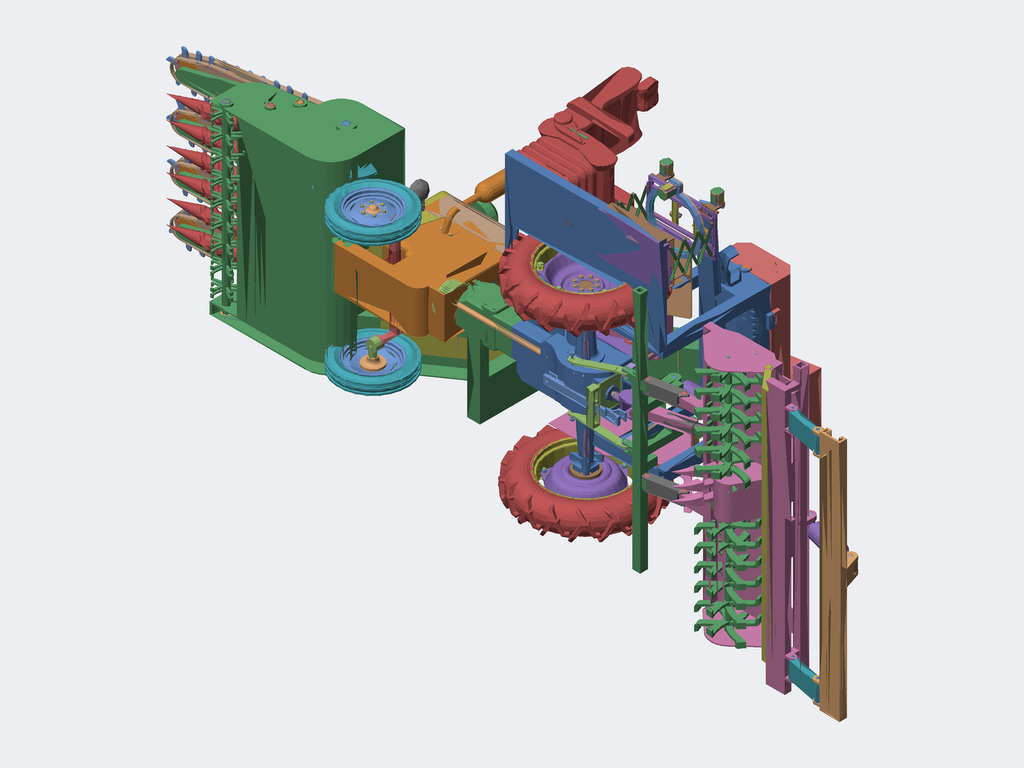Assembly | SolidWorks | 153 different items | 1051 placed
Parts list (item | name | quantity | parent item | size | volume):
1 | (subassembly) | x1 | - | - | 16381446 mm3
2 | (subassembly) | x89 | - | 79.994 x 100.305 x 21.303 mm | 62086 mm3
3 | (subassembly) | x89 | - | 59.12 x 16 x 20 mm | 6391 mm3
4 | - | x1 | - | 480 x 80 x 140 mm | 1729991 mm3
5 | - | x2 | - | 65 x 16 x 16 mm | 12827 mm3
6 | - | x2 | - | 70 x 20 x 20 mm | 21455 mm3
7 | - | x1 | - | 10 x 70 x 330 mm | 231000 mm3
8 | - | x10 | - | 25.3 x 15.011 x 13 mm | 1760 mm3
9 | - | x1 | - | 40 x 40 x 80 mm | 43982 mm3
10 | - | x2 | - | 435 x 150 x 150 mm | 3088587 mm3
11 | - | x2 | - | 380 x 110 x 110 mm | 1045872 mm3
12 | - | x1 | - | 1433 x 943.59 x 2500 mm | 127808893 mm3
13 | - | x1 | - | 50 x 305 x 2270 mm | 21360963 mm3
14 | - | x2 | - | 36 x 40 x 318 mm | 121648 mm3
15 | - | x89 | in 2 | 36.56 x 20 x 100 mm | 55695 mm3
16 | - | x1 | - | 44.721 x 70 x 40 mm | 80979 mm3
17 | - | x1 | - | 30 x 30 x 120 mm | 84731 mm3
18 | - | x1 | - | 40 x 120 x 40 mm | 150673 mm3
19 | - | x4 | - | 40 x 110 x 40 mm | 138107 mm3
20 | - | x1 | - | 50 x 150 x 50 mm | 293913 mm3
21 | - | x1 | - | 40 x 150 x 40 mm | 187421 mm3
22 | - | x4 | - | 30 x 30 x 200 mm | 141280 mm3
23 | - | x2 | - | 372 x 72 x 110 mm | 2095609 mm3
24 | - | x2 | - | 360 x 60 x 160 mm | 3106195 mm3
25 | - | x1 | - | 275 x 250 x 2300 mm | 16623350 mm3
26 | - | x2 | - | 39.6 x 34.295 x 22.3 mm | 15063 mm3
27 | - | x1 | in 1 | 25 x 25 x 230 mm | 40077 mm3
28 | - | x4 | in 1 | - | -
29 | - | x2 | in 1 | 150 x 115 x 15 mm | 137970 mm3
30 | - | x4 | in 1 | 60 x 60 x 8 mm | 18784 mm3
31 | - | x4 | in 1 | 15 x 15 x 35.5 mm | 2158 mm3
32 | - | x4 | in 1 | 60 x 10 x 10 mm | 2893 mm3
33 | - | x1 | in 1 | 605.5 x 531 x 90 mm | 1417338 mm3
34 | - | x1 | in 1 | 507.991 x 507.957 x 60 mm | 736026 mm3
35 | - | x2 | in 1 | 15 x 10 x 574 mm | 77716 mm3
36 | - | x1 | in 1 | 87.341 x 87.341 x 20 mm | 92376 mm3
37 | - | x2 | - | 130 x 50 x 50 mm | 156637 mm3
38 | - | x1 | in 1 | 634 x 120 x 390 mm | 7186342 mm3
39 | - | x1 | in 1 | 120 x 95 x 15 mm | 107220 mm3
40 | - | x1 | - | 766.626 x 1417 x 630 mm | 182133754 mm3
41 | - | x2 | in 1 | 43 x 45 x 33 mm | 8145 mm3
42 | - | x2 | in 1 | 43 x 45 x 33 mm | 8145 mm3
43 | - | x2 | in 1 | 54 x 50 x 30 mm | 26614 mm3
44 | - | x2 | in 1 | 54 x 10 x 290 mm | 145188 mm3
45 | - | x4 | in 1 | - | -
46 | - | x8 | in 1 | 32 x 12 x 33.1 mm | 9311 mm3
47 | - | x1 | - | - | -
48 | - | x2 | - | 47 x 47 x 5 mm | 6107 mm3
49 | - | x2 | in 1 | 15 x 10 x 240 mm | 32544 mm3
50 | - | x2 | in 1 | 25 x 70 x 35 mm | 25493 mm3
51 | - | x1 | in 1 | 634 x 60 x 390 mm | 1783210 mm3
52 | - | x10 | - | 82 x 50 x 50 mm | 78196 mm3
53 | - | x10 | - | 112.877 x 112.877 x 35 mm | 271354 mm3
54 | - | x20 | in 1 | 24 x 14 x 14 mm | 2187 mm3
55 | - | x2 | in 1 | 25 x 180 x 20 mm | 48842 mm3
56 | - | x1 | in 1 | 20 x 20 x 638 mm | 238279 mm3
57 | - | x12 | in 1 | 20 x 321 x 10 mm | 60985 mm3
58 | - | x12 | - | 179.981 x 179.731 x 50 mm | 415384 mm3
59 | - | x178 | in 2, 3 | 37.56 x 16 x 15 mm | 3392 mm3
60 | - | x178 | in 2, 3 | 37.56 x 16 x 20 mm | 2999 mm3
61 | - | x1 | - | 232.128 x 238.99 x 1760 mm | 6921520 mm3
62 | - | x6 | - | - | 6506170 mm3
63 | - | x1 | - | 547.5 x 225 x 360 mm | 8692071 mm3
64 | - | x1 | - | 40 x 40 x 1760 mm | 1700428 mm3
65 | - | x4 | - | 105 x 40 x 40 mm | 98226 mm3
66 | - | x1 | - | 40 x 40 x 1760 mm | 1776548 mm3
67 | - | x3 | - | 80 x 80 x 20 mm | 63234 mm3
68 | - | x1 | - | 70 x 95.558 x 40 mm | 119109 mm3
69 | - | x1 | - | 90 x 20 x 90 mm | 78186 mm3
70 | - | x4 | - | 280 x 100 x 1224 mm | 5139884 mm3
71 | - | x1 | - | 315 x 60 x 325 mm | 1362122 mm3
72 | - | x1 | - | 1005 x 380.05 x 470 mm | 23114578 mm3
73 | - | x1 | - | 1490 x 380.05 x 2280 mm | 110050960 mm3
74 | - | x1 | - | 387.638 x 226.527 x 70 mm | 165213 mm3
75 | - | x1 | - | 381.145 x 360 x 307.969 mm | 3545128 mm3
76 | - | x1 | - | 374.894 x 400 x 497.382 mm | 13317913 mm3
77 | - | x1 | - | 1005 x 791.422 x 614.545 mm | 64772988 mm3
78 | - | x2 | - | 94 x 45 x 55 mm | 48372 mm3
79 | - | x2 | - | 652 x 122 x 652 mm | 6413789 mm3
80 | - | x2 | - | 100 x 170 x 370 mm | 1067997 mm3
81 | - | x2 | - | 100 x 270 x 310 mm | 1436503 mm3
82 | - | x1 | - | 248.057 x 1018 x 150 mm | 2628075 mm3
83 | - | x1 | - | 420 x 110 x 420 mm | 545281 mm3
84 | - | x2 | - | 161 x 220.5 x 101.1 mm | 223051 mm3
85 | - | x1 | - | 153.486 x 153.486 x 325.608 mm | 831676 mm3
86 | - | x2 | - | 32.5 x 20.785 x 18 mm | 4879 mm3
87 | - | x1 | - | 510 x 325.072 x 1140 mm | 2882610 mm3
88 | - | x1 | - | 500 x 154.34 x 530 mm | 1123560 mm3
89 | - | x1 | - | 1070 x 600 x 360 mm | 4618746 mm3
90 | - | x2 | - | 244.595 x 1180 x 1180 mm | 23262229 mm3
91 | - | x2 | - | 180 x 105 x 180 mm | 867546 mm3
92 | - | x2 | - | 748.86 x 226.672 x 748.86 mm | 3116761 mm3
93 | - | x2 | - | 593.907 x 665 x 128.5 mm | 2994623 mm3
94 | - | x2 | - | 218 x 130 x 218 mm | 1192193 mm3
95 | - | x1 | - | 1070 x 600 x 360 mm | 3106000 mm3
96 | - | x2 | - | 458.731 x 420 x 1075 mm | 11323145 mm3
97 | - | x4 | - | 15 x 68 x 68 mm | 23045 mm3
98 | - | x6 | - | 12 x 60 x 60 mm | 12840 mm3
99 | - | x1 | - | 211.926 x 211.926 x 276.87 mm | 1401987 mm3
100 | - | x2 | - | 252.245 x 252.245 x 629.793 mm | 2125669 mm3
101 | - | x1 | - | 40 x 40 x 1385 mm | 1706048 mm3
102 | - | x1 | - | 209.617 x 209.617 x 100 mm | 2166914 mm3
103 | - | x2 | - | 96.667 x 455.608 x 455.608 mm | 1172743 mm3
104 | - | x1 | - | 309.756 x 309.756 x 100 mm | 4555207 mm3
105 | - | x1 | - | 435.01 x 940 x 945 mm | 125087598 mm3
106 | - | x1 | - | 530 x 40 x 400 mm | 7871394 mm3
107 | - | x1 | - | 153.486 x 153.486 x 294.64 mm | 719014 mm3
108 | - | x6 | - | 12 x 62 x 62 mm | 13593 mm3
109 | - | x1 | - | 290 x 322.5 x 290 mm | 420186 mm3
110 | - | x1 | - | 40 x 40 x 170 mm | 184147 mm3
111 | - | x1 | - | 250 x 228 x 335 mm | 4838196 mm3
112 | - | x1 | - | 490 x 137.955 x 138 mm | 3818604 mm3
113 | - | x1 | - | 12 x 42 x 42 mm | 7887 mm3
114 | - | x1 | - | 167.128 x 160.8 x 40 mm | 32904 mm3
115 | - | x1 | - | 80 x 330 x 830 mm | 1520421 mm3
116 | - | x1 | - | 70 x 218 x 225.232 mm | 296939 mm3
117 | - | x1 | - | 60 x 218 x 225.232 mm | 538282 mm3
118 | - | x2 | - | 140 x 120 x 290 mm | 1506174 mm3
119 | - | x1 | - | 1500 x 530.531 x 580 mm | 26783314 mm3
120 | - | x1 | - | 540 x 1030 x 1860 mm | 48317416 mm3
121 | - | x1 | - | 385.062 x 400 x 1200 mm | 5164108 mm3
122 | - | x1 | - | 4060 x 1991 x 1785 mm | 166702923 mm3
123 | - | x1 | - | 480.011 x 480.011 x 1760 mm | 34687851 mm3
124 | - | x6 | - | 7 x 65 x 65 mm | 6140 mm3
125 | - | x4 | - | 7 x 32 x 32 mm | 2319 mm3
126 | - | x2 | - | 40 x 40 x 415 mm | 466608 mm3
127 | - | x1 | - | 710 x 70 x 85 mm | 1467586 mm3
128 | - | x2 | - | 255 x 41.569 x 36 mm | 118287 mm3
129 | - | x2 | - | 55 x 140 x 140 mm | 524256 mm3
130 | - | x2 | - | 24 x 2.5 x 24 mm | 784.672 mm3
131 | - | x2 | - | 37 x 3 x 37 mm | 2154 mm3
132 | - | x10 | - | 20 x 2 x 20 mm | 427.568 mm3
133 | - | x4 | - | 77.7 x 43 x 43 mm | 30766 mm3
134 | - | x4 | - | 25.5 x 17.5 x 17.5 mm | 2396 mm3
135 | - | x12 | - | 23.7 x 23.7 x 3 mm | 898.415 mm3
136 | - | x12 | - | 18 x 20.785 x 12 mm | 2348 mm3
137 | - | x28 | - | 38.4 x 38.4 x 4 mm | 3151 mm3
138 | - | x16 | - | 24 x 27.713 x 16.4 mm | 5589 mm3
139 | - | x2 | - | 510.518 x 105 x 65 mm | 489274 mm3
140 | - | x1 | - | 480 x 80 x 140 mm | 1449991 mm3
141 | - | x14 | - | 33 x 28.579 x 19 mm | 8913 mm3
142 | - | x12 | - | 92.5 x 34.641 x 30 mm | 34747 mm3
143 | - | x4 | - | 70 x 70 x 30 mm | 65058 mm3
144 | - | x1 | - | 510 x 622 x 2300 mm | 17041991 mm3
145 | - | x1 | - | 100 x 99.955 x 305 mm | 1401130 mm3
146 | - | x1 | - | 180 x 165 x 210 mm | 1913564 mm3
147 | - | x2 | - | 150 x 20 x 150 mm | 232085 mm3
148 | - | x2 | - | 70 x 70 x 20 mm | 49524 mm3
149 | - | x2 | - | 52.5 x 34.641 x 30 mm | 22112 mm3
150 | - | x2 | - | 387.698 x 79.396 x 190 mm | 762316 mm3
151 | - | x1 | - | 593 x 758 x 290 mm | 1986947 mm3
152 | plain washers--product grade c gb | x1 | - | - | -
153 | prevailing torque all-metal 1 gb | x1 | - | - | -
Mates (type | each side: item.copy, entity, surface, feature), first 556 of 812 lines:
In the top assembly
Coincident | 73.1 face plane Boss-Extrude 1 | 77.1 face plane Boss-Extrude 1 | 2 times
Coincident | 73.1 face plane Cut-Extrude 1 | 77.1 face plane Boss-Extrude 1
Coincident | 105.1 face plane Cut-Extrude 1 | 77.1 face plane Boss-Extrude 7 | 2 times
Coincident | 105.1 edge | 77.1 face plane Boss-Extrude 7
Concentric | 105.1 face cylinder Boss-Extrude 11 | 115.1 face cylinder Boss-Extrude 2
Coincident | 105.1 face plane Boss-Extrude 1 | 115.1 face plane Boss-Extrude 2
Parallel | 105.1 face plane Boss-Extrude 13 | 115.1 face plane Extrude-Thin 3
Coincident | 73.1 face plane Boss-Extrude 1 | 63.1 face plane Boss-Extrude 1
Coincident | 73.1 face plane Boss-Extrude 1 | 63.1 face plane Boss-Extrude 3 | 2 times
Coincident | 73.1 face plane Boss-Extrude 1 | 75.1 face plane Boss-Extrude 2
Coincident | 73.1 face plane Cut-Extrude 1 | 75.1 face plane Boss-Extrude 2
Coincident | 63.1 face plane Boss-Extrude 1 | 75.1 face plane Boss-Extrude 2
Width | 76.1 face plane Boss-Extrude 4 | 76.1 face plane Boss-Extrude 4 | 63.1 face plane Mirror 2 | 63.1 face plane Boss-Extrude 2
Coincident | 63.1 face plane Boss-Extrude 1 | 76.1 face plane Boss-Extrude 4 | 2 times
Concentric | 105.1 face cylinder Boss-Extrude 4 | 106.1 face cylinder Cut-Extrude 3
Coincident | 105.1 face plane Boss-Extrude 3 | 106.1 face plane Cut-Extrude 4
LimitPlanarAngleDim | 105.1 face plane Boss-Extrude 1 | 106.1 face plane Boss-Extrude 1
Concentric | 91.1 face cylinder Revolve 1 | 103.1 face cylinder Thicken 2
Concentric | 91.1 face cylinder Boss-Extrude 1 | 103.1 face cylinder Cut-Extrude 1
Coincident | 91.1 face plane Revolve 1 | 103.1 face plane Thicken 2
Concentric | 79.1 face cylinder Thicken 1 | 103.1 face cylinder Thicken 1
Width | 103.1 face plane Thicken 1 | 103.1 face plane Thicken 1 | 79.1 face plane Thicken 1 | 79.1 face plane Thicken 1
Concentric | 80.1 face cylinder Boss-Extrude 3 | 81.1 face cylinder Cut-Extrude 1
Coincident | 80.1 edge | 81.1 face plane Revolve 1
Coincident | 91.1 face plane Revolve 1 | 80.1 face plane Boss-Extrude 1
Concentric | 91.1 face cylinder Revolve 1 | 80.1 face cylinder Boss-Extrude 1
Concentric | 115.1 face cylinder Extrude-Thin 1 | 81.1 face cylinder Boss-Extrude 1
LimitDistanceDim | 81.1 face plane Boss-Extrude 1 | 115.1 face plane Extrude-Thin 1
Parallel | 105.1 face plane Boss-Extrude 13 | 80.1 face plane Boss-Extrude 3
Coincident | 77.1 edge | 83.1 face plane CirPattern 1
Concentric | 77.1 face cylinder Boss-Extrude 6 | 83.1 face cylinder CirPattern 1
Coincident | 151.1 face plane Boss-Extrude 1 | 87.1 face plane Boss-Extrude 1
Concentric | 151.1 face cylinder Fillet 2 | 87.1 face cylinder Boss-Extrude 1
Coincident | 151.1 face plane Cut-Extrude 1 | 87.1 face plane Boss-Extrude 1
Concentric | 87.1 face cylinder Boss-Extrude 1 | 88.1 face cylinder Fillet 1 | 2 times
Coincident | 87.1 face plane Boss-Extrude 1 | 88.1 face plane Boss-Extrude 1
Width | 88.1 face plane Boss-Extrude 1 | 88.1 face plane Boss-Extrude 1 | 73.1 face plane Cut-Extrude 1 | 73.1 face plane Mirror 1
Coincident | 88.1 face plane Cut-Extrude 4 | 73.1 face plane Boss-Extrude 1
Coincident | 75.1 face plane Boss-Extrude 2 | 88.1 edge
Parallel | 105.1 face plane Boss-Extrude 1 | 91.1 face plane Revolve 1
Concentric | 81.2 face cylinder Revolve 1 | 80.2 face cylinder Boss-Extrude 3
Coincident | 81.2 face plane Revolve 1 | 80.2 face plane Boss-Extrude 2
Concentric | 115.1 face cylinder Extrude-Thin 1 | 81.2 face cylinder Boss-Extrude 1
LimitDistanceDim | 115.1 face plane Extrude-Thin 1 | 81.2 face plane Boss-Extrude 1
Parallel | 105.1 face plane Boss-Extrude 13 | 80.2 face plane Boss-Extrude 3
Concentric | 80.2 face cylinder Boss-Extrude 1 | 91.2 face cylinder Revolve 1
Coincident | 80.2 face plane Boss-Extrude 1 | 91.2 face plane Revolve 1
Parallel | 105.1 face plane Boss-Extrude 1 | 91.2 face plane Revolve 1
Concentric | 103.2 edge | 91.2 face cylinder Revolve 1
Concentric | 103.2 face cylinder CirPattern 1 | 91.2 face cylinder CirPattern 1
Coincident | 103.2 face plane Thicken 2 | 91.2 face plane Revolve 1
Width | 103.2 face plane Thicken 1 | 103.2 face plane Thicken 1 | 79.2 face plane Thicken 1 | 79.2 face plane Thicken 1
Concentric | 79.2 face cylinder Thicken 1 | 103.2 face cylinder Thicken 1
Concentric | 105.1 edge | 82.1 face cylinder Boss-Extrude 2
Coincident | 105.1 edge | 82.1 face cylinder Boss-Extrude 2
Coincident | 105.1 face plane Boss-Extrude 1 | 82.1 face plane Boss-Extrude 2
Concentric | 105.1 face cylinder Cut-Extrude 14 | 109.1 face cylinder Boss-Extrude 1 | 2 times
Coincident | 105.1 face plane Boss-Extrude 7 | 109.1 face plane Boss-Extrude 1
Concentric | 93.1 face cylinder Thicken 1 | 94.1 edge
Coincident | 93.1 face plane Thicken 1 | 94.1 face plane Revolve 1
Concentric | 93.1 face cylinder CirPattern 2 | 94.1 face cylinder CirPattern 1
Concentric | 94.2 face cylinder Revolve 1 | 93.2 face cylinder Thicken 1
Coincident | 94.2 face plane Revolve 1 | 93.2 face plane Thicken 1
Concentric | 94.2 face cylinder CirPattern 1 | 93.2 face cylinder CirPattern 2
Coincident | 94.1 face plane Boss-Extrude 2 | 100.1 face plane Cut-Extrude 1
Concentric | 94.1 face cylinder Revolve 1 | 100.1 face cylinder Boss-Extrude 1
Coincident | 94.1 face plane Revolve 1 | 100.1 face plane Boss-Extrude 1
Concentric | 94.2 face cylinder Revolve 1 | 100.2 face cylinder Boss-Extrude 1
Coincident | 94.2 face plane Boss-Extrude 2 | 100.2 face plane Cut-Extrude 1
Coincident | 94.2 face plane Revolve 1 | 100.2 edge
Concentric | 73.1 face cylinder Cut-Extrude 2 | 100.2 face cylinder Boss-Extrude 1
Concentric | 73.1 face cylinder Cut-Extrude 2 | 100.1 face cylinder Boss-Extrude 1
Concentric | 98.1 face cylinder Boss-Revolve 4 | 98.2 face cylinder Boss-Revolve 4
Concentric | 100.1 face cylinder Boss-Extrude 1 | 98.2 face cylinder Boss-Revolve 4
Coincident | 100.1 face plane Boss-Extrude 3 | 98.1 face plane Mirror All 1
Coincident | 100.1 face plane Boss-Extrude 2 | 98.2 face plane Boss-Revolve 4
Concentric | 98.3 face cylinder Boss-Revolve 4 | 98.4 face cylinder Boss-Revolve 4
Concentric | 100.2 face cylinder Boss-Extrude 1 | 98.4 face cylinder Boss-Revolve 3
Coincident | 100.2 edge | 98.3 face plane Boss-Revolve 4
Coincident | 100.2 face plane Boss-Extrude 2 | 98.4 edge
Coincident | 73.1 face plane Mirror 1 | 94.2 face plane Revolve 1
Coincident | 73.1 face plane Boss-Extrude 10 | 94.1 face plane Revolve 1
Concentric | 73.1 face cylinder Cut-Extrude 6 | 99.1 face cylinder Boss-Extrude 1
Concentric | 73.1 face cylinder Boss-Extrude 15 | 97.1 face cylinder Boss-Revolve 4
Coincident | 73.1 face plane Shell 1 | 97.1 face plane Mirror All 1
Coincident | 99.1 face plane Cut-Extrude 1 | 101.1 face plane Boss-Extrude 5 | 2 times
Concentric | 99.1 face cylinder Cut-Extrude 1 | 101.1 face cylinder Boss-Extrude 2
Concentric | 101.1 face cylinder Boss-Extrude 2 | 97.2 face cylinder Boss-Revolve 3
Coincident | 77.1 face plane Cut-Extrude 3 | 97.2 face plane Mirror All 1
Concentric | 101.1 face cylinder Boss-Extrude 2 | 98.5 face cylinder Boss-Revolve 3
Coincident | 105.1 edge | 98.5 face plane Mirror All 1
Concentric | 105.1 face cylinder Cut-Extrude 16 | 98.6 face cylinder Mirror All 1
Coincident | 105.1 face plane Extrude-Thin 3 | 98.6 face plane Mirror All 1
Concentric | 105.1 face cylinder Cut-Extrude 16 | 98.6 face cylinder Boss-Revolve 4
Coincident | 101.1 face plane Boss-Extrude 3 | 104.1 face plane Cut-Extrude 2
Concentric | 101.1 face cylinder Boss-Extrude 2 | 104.1 face cylinder Cut-Extrude 2
Coincident | 101.1 edge | 104.1 face plane SpurGear2
Concentric | 105.1 face cylinder Boss-Extrude 6 | 102.1 face cylinder Cut-Extrude 1
Coincident | 102.1 face plane SpurGear1 | 104.1 face plane SpurGear2
GearDim | 104.1 edge | 102.1 edge
Concentric | 108.1 face cylinder Boss-Revolve 4 | 108.2 face cylinder Boss-Revolve 4
Coincident | 102.1 face plane Cut-Extrude 1 | 108.2 face plane Boss-Revolve 4
Concentric | 102.1 face cylinder Cut-Extrude 1 | 108.2 face cylinder Boss-Revolve 3
Coincident | 102.1 face plane SpurGear1 | 108.1 face plane Boss-Revolve 3
Coincident | 105.1 face plane Boss-Extrude 6 | 102.1 face plane Cut-Extrude 1
Concentric | 111.1 face cylinder Cut-Extrude 5 | 112.1 face cylinder Revolve 1
Coincident | 111.1 face plane Boss-Extrude 3 | 112.1 face plane Revolve 1
Concentric | 112.1 face cylinder Revolve 1 | 113.1 face cylinder Boss-Revolve 4
Coincident | 111.1 face plane Boss-Extrude 1 | 113.1 face plane Boss-Revolve 4
Concentric | 112.1 face cylinder Revolve 1 | 114.1 face cylinder Boss-Extrude 1
Coincident | 112.1 face plane Cut-Extrude 3 | 114.1 face plane Boss-Extrude 3
Coincident | 112.1 face plane Revolve 1 | 114.1 face plane Boss-Extrude 2
Concentric | 111.1 face cylinder Boss-Extrude 1 | 116.1 face cylinder Thicken 1
Concentric | 111.1 face cylinder CirPattern 2 | 116.1 face cylinder CirPattern 1
Coincident | 111.1 face plane Boss-Extrude 1 | 116.1 face plane Thicken 1
Concentric | 111.1 face cylinder Boss-Extrude 1 | 117.1 face cylinder Thicken 1
Concentric | 111.1 face cylinder CirPattern 3 | 117.1 face cylinder CirPattern 4
Coincident | 111.1 face plane Boss-Extrude 1 | 117.1 face plane Thicken 1
Concentric | 98.6 face cylinder Boss-Revolve 4 | 112.1 face cylinder Revolve 1
Parallel | 105.1 face plane Boss-Extrude 2 | 111.1 face plane Boss-Extrude 2
Concentric | 112.1 face cylinder Revolve 1 | 110.1 face cylinder Boss-Extrude 1
Coincident | 112.1 face plane Cut-Extrude 4 | 110.1 face plane Boss-Extrude 3
Coincident | 112.1 face plane Revolve 1 | 110.1 edge
Concentric | 102.1 face cylinder Cut-Extrude 2 | 110.1 face cylinder Boss-Extrude 1
Coincident | 102.1 face plane Cut-Extrude 2 | 110.1 face plane Boss-Extrude 1 | 2 times
GearDim | 100.1 edge | 99.1 edge
GearDim | 99.1 edge | 100.2 edge
Concentric | 151.1 face cylinder Mirror 7 | 84.1 face cylinder Boss-Extrude 3
Coincident | 151.1 face plane Boss-Extrude 1 | 84.1 face plane Boss-Extrude 3
Parallel | 105.1 face plane Boss-Extrude 1 | 84.1 plane
Concentric | 151.1 face cylinder Boss-Extrude 3 | 84.2 face cylinder Shell 2
Coincident | 151.1 face plane Boss-Extrude 1 | 84.2 face plane Boss-Extrude 3
Parallel | 105.1 face plane Boss-Extrude 1 | 84.2 plane
Coincident | 73.1 face plane Boss-Extrude 11 | 89.1 face plane Boss-Extrude 1
Coincident | 73.1 face plane Boss-Extrude 11 | 89.1 face plane Boss-Extrude 2
Coincident | 73.1 face plane Mirror 1 | 95.1 face plane Boss-Extrude 1 | 2 times
Tangent | 73.1 face cylinder Mirror 1 | 95.1 face plane Boss-Extrude 5
Coincident | 93.1 face plane Thicken 1 | 92.1 face plane Thicken 2
Concentric | 93.1 face cylinder CirPattern 1 | 92.1 face cylinder Cut-Extrude 1
Concentric | 93.1 face cone Thicken 1 | 92.1 face cylinder Thicken 1
Concentric | 90.1 face cylinder Mirror 1 | 92.1 face cylinder Thicken 1
Width | 90.1 face plane Thicken 1 | 90.1 face plane Mirror 1 | 92.1 face plane Thicken 1 | 92.1 face plane Thicken 1
Concentric | 90.2 face cylinder Thicken 1 | 92.2 face cylinder Thicken 1
Concentric | 93.2 face cone Thicken 1 | 92.2 face cylinder Thicken 1
Concentric | 93.2 face cylinder CirPattern 1 | 92.2 face cylinder CirPattern 4
Coincident | 93.2 face plane Thicken 1 | 92.2 face plane CirPattern 4
Width | 92.2 face plane Thicken 1 | 92.2 face plane Thicken 1 | 90.2 face plane Mirror 1 | 90.2 face plane Thicken 1
Coincident | 149.1 face plane Base-Extrude | 149.2 face plane Base-Extrude
Concentric | 109.1 face cylinder Boss-Extrude 1 | 149.1 face cylinder Boss-Revolve 1
Concentric | 109.1 face cylinder Boss-Extrude 1 | 149.2 face cylinder Boss-Revolve 1
Concentric | 82.1 face cylinder Boss-Extrude 2 | 86.1 face cylinder Boss-Revolve 1
Concentric | 82.1 face cylinder Boss-Extrude 2 | 86.2 face cylinder Boss-Revolve 1
Coincident | 86.1 face plane Base-Extrude | 86.2 face plane Base-Extrude
Concentric | 116.1 face cylinder Cut-Extrude 1 | 8.1 face cylinder Boss-Revolve 1
Concentric | 117.1 face cylinder CirPattern 4 | 8.2 face cylinder Boss-Revolve 1
Concentric | 63.1 face cylinder Boss-Extrude 1 | 150.1 face cylinder Boss-Extrude 4
Coincident | 63.1 face plane Boss-Extrude 1 | 150.1 face plane Boss-Extrude 2
Concentric | 150.1 face cylinder Boss-Extrude 1 | 14.1 face cylinder Extrude-Thin 1
Coincident | 150.1 face plane Cut-Extrude 1 | 14.1 face plane Extrude-Thin 1
Coincident | 37.1 face plane Boss-Extrude 2 | 14.1 face plane Boss-Extrude 1
Concentric | 37.1 face cylinder Boss-Extrude 2 | 14.1 face cylinder Boss-Extrude 1
Concentric | 73.1 face cylinder Boss-Extrude 12 | 139.1 face cylinder Cut-Extrude 1
Concentric | 139.1 face cylinder Cut-Extrude 1 | 37.1 face cylinder Cut-Extrude 2
Width | 139.1 face plane Boss-Extrude 2 | 139.1 face plane Boss-Extrude 2 | 37.1 face plane Cut-Extrude 1 | 37.1 face plane Cut-Extrude 1
Concentric | 14.2 face cylinder Extrude-Thin 1 | 150.2 face cylinder Boss-Extrude 1
Coincident | 14.2 face plane Extrude-Thin 1 | 150.2 face plane Cut-Extrude 1
Concentric | 37.2 face cylinder Boss-Extrude 2 | 14.2 face cylinder Boss-Extrude 1
Coincident | 37.2 face plane Boss-Extrude 2 | 14.2 face plane Boss-Extrude 1
Concentric | 139.2 face cylinder Cut-Extrude 1 | 37.2 face cylinder Cut-Extrude 2
Width | 139.2 face plane Boss-Extrude 2 | 139.2 face plane Boss-Extrude 2 | 37.2 face plane Cut-Extrude 1 | 37.2 face plane Cut-Extrude 1
Concentric | 63.1 face cylinder Boss-Extrude 1 | 150.2 face cylinder Boss-Extrude 4
Coincident | 63.1 face plane Boss-Extrude 1 | 150.2 face plane Boss-Extrude 2
Concentric | 73.1 face cylinder Mirror 1 | 139.2 face cylinder Cut-Extrude 1
Concentric | 37.1 face cylinder Cut-Extrude 2 | 37.2 face cylinder Cut-Extrude 2
Coincident | 120.1 edge | 97.3 face cylinder Boss-Revolve 3
Coincident | 120.1 face plane Shell 2 | 97.3 face plane Boss-Revolve 4
Concentric | 97.3 face cylinder Boss-Revolve 4 | 97.4 face cylinder Boss-Revolve 4
Coincident | 120.1 face plane Shell 2 | 97.4 face plane Mirror All 1
Concentric | 121.1 face cylinder Boss-Extrude 2 | 97.4 face cylinder Boss-Revolve 4
Coincident | 120.1 face plane Boss-Extrude 18 | 121.1 face plane Boss-Extrude 2
Coincident | 73.1 face plane Boss-Extrude 18 | 120.1 face plane Boss-Extrude 10
Coincident | 73.1 face plane Mirror 2 | 120.1 face plane Cut-Extrude 4 | 2 times
Coincident | 105.1 face plane Boss-Extrude 1 | 122.1 face plane Cut-Extrude 18
Coincident | 105.1 face plane Cut-Extrude 19 | 122.1 face plane Cut-Extrude 21
Coincident | 105.1 face plane Boss-Extrude 13 | 122.1 face plane Cut-Extrude 21
Concentric | 122.1 face cylinder Cut-Extrude 15 | 125.1 face cylinder Boss-Revolve 3
Coincident | 122.1 face plane Mirror 2 | 125.1 face plane Mirror All 1
Concentric | 125.1 face cylinder Boss-Revolve 4 | 125.2 face cylinder Boss-Revolve 4
Coincident | 122.1 face plane Cut-Extrude 16 | 125.2 face plane Mirror All 1
Concentric | 125.3 face cylinder Boss-Revolve 4 | 125.4 face cylinder Boss-Revolve 4
Concentric | 122.1 face cylinder Mirror 3 | 125.3 face cylinder Boss-Revolve 4
Coincident | 122.1 face plane Boss-Extrude 8 | 125.4 face plane Boss-Revolve 4
Coincident | 122.1 edge | 125.3 face plane Mirror All 1
Coincident | 122.1 edge | 124.1 face cylinder Boss-Revolve 3
Coincident | 122.1 face plane Boss-Extrude 7 | 124.1 face plane Boss-Revolve 3
Concentric | 122.1 face cylinder Cut-Extrude 11 | 124.2 face cylinder Boss-Revolve 4
Coincident | 122.1 face plane Mirror 1 | 124.2 face plane Boss-Revolve 3
Concentric | 124.3 face cylinder Boss-Revolve 4 | 124.4 face cylinder Boss-Revolve 4
Concentric | 122.1 edge | 124.4 face cylinder Boss-Revolve 4
Coincident | 122.1 face plane Cut-Extrude 12 | 124.3 face plane Boss-Revolve 3
Coincident | 122.1 face plane Boss-Extrude 6 | 124.4 face plane Boss-Revolve 4
Concentric | 146.1 face cylinder Boss-Extrude 1 | 145.1 face cylinder Revolve 1
Width | 145.1 face plane Revolve 1 | 145.1 face plane Revolve 1 | 146.1 face plane Cut-Extrude 4 | 146.1 face plane Mirror 1
Concentric | 145.1 face cylinder Boss-Extrude 1 | 147.1 face cylinder Cut-Extrude 1
Concentric | 146.1 face cylinder Boss-Extrude 1 | 147.2 face cylinder Revolve 1
Coincident | 146.1 face plane Cut-Extrude 5 | 147.2 face plane Cut-Extrude 2
Coincident | 146.1 face plane Mirror 2 | 147.1 face plane Cut-Extrude 2
Coincident | 95.1 face plane Boss-Extrude 1 | 146.1 face plane Boss-Extrude 2
Coincident | 95.1 edge | 146.1 edge
Coincident | 145.1 face plane Cut-Extrude 1 | 148.1 face plane Cut-Extrude 1
Concentric | 145.1 face cylinder Boss-Extrude 1 | 148.1 face cylinder Cut-Extrude 1
Coincident | 145.1 face plane Boss-Extrude 1 | 148.1 face plane Boss-Extrude 1
Coincident | 121.1 face plane Boss-Extrude 3 | 148.1 face plane Boss-Extrude 1
Concentric | 121.1 face cylinder Boss-Extrude 3 | 148.2 face cylinder Cut-Extrude 1
Coincident | 121.1 face plane Boss-Extrude 3 | 148.2 face plane Boss-Extrude 1
Coincident | 121.1 face plane Cut-Extrude 1 | 148.2 face plane Cut-Extrude 1
Concentric | 122.1 face cylinder Cut-Extrude 11 | 123.1 face cylinder Boss-Extrude 1
Coincident | 122.1 face plane Mirror 1 | 123.1 face plane Boss-Extrude 1
Concentric | 125.1 edge | 126.1 face cylinder Boss-Extrude 1
Coincident | 122.1 face plane Mirror 1 | 126.1 face plane Boss-Extrude 1
Concentric | 122.1 face cylinder Cut-Extrude 15 | 126.2 face cylinder Boss-Extrude 1
Coincident | 122.1 face plane Mirror 1 | 126.2 face plane Boss-Extrude 1
Concentric | 73.1 face cylinder Boss-Extrude 3 | 71.1 face cylinder Boss-Extrude 1
Coincident | 73.1 face plane Boss-Extrude 2 | 71.1 face plane Boss-Extrude 1 | 2 times
Width | 127.1 face plane Boss-Extrude 1 | 127.1 face plane Boss-Extrude 1 | 71.1 face plane Boss-Extrude 2 | 71.1 face plane Boss-Extrude 2
Coincident | 127.1 face plane Boss-Extrude 1 | 71.1 face plane Boss-Extrude 2
Concentric | 145.1 face cylinder Boss-Extrude 1 | 143.1 face cylinder Boss-Extrude 1
Coincident | 145.1 face plane Boss-Extrude 1 | 143.1 face plane Boss-Extrude 1
Coincident | 145.1 face plane Cut-Extrude 2 | 143.1 face plane Boss-Extrude 1
Concentric | 126.1 face cylinder Boss-Extrude 4 | 143.2 face cylinder Boss-Extrude 1
Coincident | 126.1 face plane Cut-Extrude 2 | 143.2 face plane Boss-Extrude 1
Coincident | 126.1 face plane Boss-Extrude 2 | 143.2 face plane Boss-Extrude 1
Concentric | 126.2 face cylinder Boss-Extrude 4 | 143.3 face cylinder Boss-Extrude 1
Coincident | 126.2 face plane Cut-Extrude 2 | 143.3 face plane Boss-Extrude 1
Coincident | 126.2 face plane Boss-Extrude 2 | 143.3 face plane Boss-Extrude 1
Concentric | 123.1 face cylinder Cut-Extrude 1 | 143.4 face cylinder Boss-Extrude 1
Coincident | 143.3 face plane Boss-Extrude 1 | 143.4 face plane Boss-Extrude 1
Coincident | 123.1 face plane Cut-Extrude 2 | 143.4 face plane Boss-Extrude 1
Coincident | 95.1 face plane Cut-Extrude 1 | 78.1 face plane Boss-Extrude 1 | 2 times
Coincident | 95.1 face plane Boss-Extrude 1 | 78.1 face plane Boss-Extrude 1
Coincident | 89.1 face plane Boss-Extrude 1 | 78.2 face plane Boss-Extrude 1
Coincident | 89.1 face plane Cut-Extrude 1 | 78.2 face plane Boss-Extrude 1 | 2 times
BeltDim | 148.2 face cylinder Cut-Revolve 1 | 148.1 face cylinder Cut-Revolve 1
BeltDim | 143.1 face cylinder Cut-Revolve 1 | 143.2 face cylinder Cut-Revolve 1
BeltDim | 143.3 face cylinder Cut-Revolve 1 | 143.4 face cylinder Cut-Revolve 1
Concentric | 73.1 face cylinder Size mm Dowel Hole 1 | 144.1 face cylinder Cut-Extrude 6 | 2 times
Width | 144.1 face plane Boss-Extrude 3 | 144.1 face plane Boss-Extrude 3 | 73.1 face plane Mirror 1 | 73.1 face plane Boss-Extrude 7
Concentric | 9.1 face cylinder Boss-Extrude 1 | 10.1 face cylinder Boss-Extrude 1
Concentric | 144.1 face cylinder Cut-Extrude 5 | 9.1 face cylinder Boss-Extrude 1
Coincident | 144.1 face plane Cut-Extrude 4 | 9.1 face plane Boss-Extrude 1
Coincident | 144.1 face plane Cut-Extrude 4 | 10.1 face plane Boss-Extrude 1
Concentric | 10.1 face cylinder Revolve 3 | 11.1 face cylinder Revolve 1
LimitDistanceDim | 10.1 face plane Revolve 3 | 11.1 face plane Revolve 1
Concentric | 11.1 face cylinder Boss-Extrude 1 | 12.1 face cylinder Cut-Extrude 10
Coincident | 11.1 face plane Boss-Extrude 1 | 12.1 face plane Cut-Extrude 9
Concentric | 12.1 face cylinder Cut-Extrude 2 | 23.1 face cylinder Boss-Extrude 1
Concentric | 12.1 face cylinder Cut-Extrude 2 | 23.2 face cylinder Boss-Extrude 1
Concentric | 12.1 face cylinder Cut-Extrude 11 | 13.1 face cylinder Boss-Extrude 1
Coincident | 12.1 face plane Boss-Extrude 1 | 13.1 face plane Boss-Extrude 1
LimitPlanarAngleDim | 13.1 face plane Boss-Extrude 2 | 12.1 face plane Boss-Extrude 5
Concentric | 12.1 face cylinder Cut-Extrude 17 | 24.1 face cylinder Boss-Extrude 1
Coincident | 12.1 face plane Cut-Extrude 16 | 24.1 face plane Boss-Extrude 1
Concentric | 12.1 face cylinder Mirror 6 | 24.2 face cylinder Boss-Extrude 1
Coincident | 12.1 face plane Mirror 6 | 24.2 face plane Boss-Extrude 1
Concentric | 24.1 face cylinder Boss-Extrude 1 | 25.1 face cylinder Cut-Extrude 4
Coincident | 24.1 face plane Boss-Extrude 1 | 25.1 face plane Cut-Extrude 3
Concentric | 11.2 face cylinder Boss-Extrude 1 | 25.1 face cylinder Boss-Extrude 5
Coincident | 25.1 face plane Cut-Extrude 2 | 11.2 face plane Boss-Extrude 1
Concentric | 12.1 face cylinder Cut-Extrude 15 | 10.2 face cylinder Boss-Extrude 1
Coincident | 12.1 face plane Cut-Extrude 14 | 10.2 face plane Boss-Extrude 1
Concentric | 10.2 face cylinder Revolve 3 | 11.2 face cylinder Revolve 1
Concentric | 24.2 face cylinder Boss-Extrude 1 | 25.1 face cylinder Mirror 1
Concentric | 144.1 face cylinder Cut-Extrude 5 | 17.1 face cylinder Boss-Extrude 1
Coincident | 144.1 face plane Boss-Extrude 5 | 17.1 face plane Boss-Extrude 1
Concentric | 12.1 face cylinder Cut-Extrude 10 | 18.1 face cylinder Revolve 1
Coincident | 12.1 face plane Boss-Extrude 3 | 18.1 face plane Revolve 1
Coincident | 23.1 face plane Boss-Extrude 1 | 19.1 face plane Revolve 1
Coincident | 23.1 face plane Boss-Extrude 1 | 19.2 face plane Revolve 1
Concentric | 12.1 face cylinder Cut-Extrude 2 | 19.2 face cylinder Revolve 1
Coincident | 23.2 face plane Boss-Extrude 1 | 19.3 face plane Revolve 1
Concentric | 12.1 face cylinder Cut-Extrude 2 | 19.4 face cylinder Revolve 1
Coincident | 23.2 face plane Boss-Extrude 1 | 19.4 face plane Revolve 1
Concentric | 10.2 face cylinder Boss-Extrude 1 | 20.1 face cylinder Revolve 1
Coincident | 12.1 face plane Boss-Extrude 13 | 20.1 face plane Revolve 1
Concentric | 11.2 face cylinder Boss-Extrude 1 | 21.1 face cylinder Revolve 1
Coincident | 25.1 face plane Boss-Extrude 5 | 21.1 face plane Revolve 1
Concentric | 24.1 face cylinder Boss-Extrude 1 | 22.1 face cylinder Boss-Extrude 1
Coincident | 12.1 face plane Boss-Extrude 14 | 22.1 face plane Boss-Extrude 1
Concentric | 24.2 face cylinder Boss-Extrude 1 | 22.2 face cylinder Boss-Extrude 1
Coincident | 12.1 face plane Mirror 6 | 22.2 face plane Boss-Extrude 1
Concentric | 24.2 face cylinder Boss-Extrude 1 | 22.3 face cylinder Boss-Extrude 1
Coincident | 25.1 face plane Mirror 1 | 22.3 face plane Boss-Extrude 1
Concentric | 24.1 face cylinder Boss-Extrude 1 | 22.4 face cylinder Boss-Extrude 1
Coincident | 25.1 face plane Boss-Extrude 6 | 22.4 face plane Boss-Extrude 1
LimitPlanarAngleDim | 23.1 face plane Boss-Extrude 1 | 144.1 face plane Boss-Extrude 1
Parallel | 144.1 face plane Boss-Extrude 1 | 12.1 face plane Boss-Extrude 1
LimitPlanarAngleDim | 24.1 face plane Boss-Extrude 1 | 12.1 face plane Boss-Extrude 11
Parallel | 12.1 face plane Boss-Extrude 11 | 25.1 face plane Boss-Extrude 1
LimitPlanarAngleDim | 24.1 face plane Boss-Extrude 1 | 25.1 face plane Boss-Extrude 1
Concentric | 12.1 face cylinder Boss-Extrude 17 | 85.1 face cylinder Boss-Extrude 1
Coincident | 12.1 face plane Boss-Extrude 17 | 85.1 face plane Boss-Extrude 5
Concentric | 12.1 face cylinder Cut-Extrude 19 | 96.1 face cylinder Boss-Extrude 1
Coincident | 12.1 face plane Shell 1 | 96.1 face plane Boss-Extrude 2
GearDim | 96.1 edge | 85.1 edge
Concentric | 12.1 face cylinder Cut-Extrude 19 | 96.2 face cylinder Boss-Extrude 1
Coincident | 12.1 face plane Shell 1 | 96.2 face plane Boss-Extrude 2
GearDim | 85.1 edge | 96.2 edge
Concentric | 12.1 face cylinder Cut-Extrude 23 | 107.1 face cylinder Boss-Extrude 1
GearDim | 107.1 edge | 85.1 edge
Coincident | 12.1 face plane Shell 1 | 107.1 face plane Boss-Extrude 2
Concentric | 99.1 face cylinder Boss-Extrude 2 | 118.1 face cylinder Cut-Extrude 3
Coincident | 99.1 face plane Boss-Extrude 2 | 118.1 face plane Cut-Extrude 3
Coincident | 99.1 face plane Boss-Extrude 2 | 118.1 face plane Boss-Extrude 1
Parallel | 90.1 select_type:24 | 93.1 select_type:24
Parallel | 93.2 select_type:24 | 90.2 select_type:24
Parallel | 79.2 select_type:24 | 103.2 select_type:24
Parallel | 79.1 select_type:24 | 103.1 select_type:24
Concentric | 107.1 face cylinder Boss-Extrude 1 | 118.2 face cylinder Boss-Extrude 1
Parallel | 107.1 face plane Boss-Extrude 3 | 118.2 face plane Cut-Extrude 3
Coincident | 107.1 face plane Boss-Extrude 3 | 118.2 face plane Boss-Extrude 1
Concentric | 118.1 face cylinder Cut-Extrude 4 | 129.1 face cylinder Revolve 1
Coincident | 118.1 face plane Boss-Extrude 2 | 129.1 face plane Revolve 1
Concentric | 118.2 face cylinder Cut-Extrude 4 | 129.2 face cylinder Revolve 1
Coincident | 118.2 face plane Boss-Extrude 2 | 129.2 face plane Revolve 1
Concentric | 129.1 face cylinder Boss-Extrude 1 | 140.1 face cylinder Boss-Extrude 1
Coincident | 129.1 face plane Boss-Extrude 1 | 140.1 face plane Boss-Extrude 1
Coincident | 140.1 face plane Cut-Extrude 2 | 4.1 face plane Boss-Extrude 3 | 2 times
Concentric | 129.2 face cylinder Boss-Extrude 1 | 4.1 face cylinder Boss-Extrude 1
Coincident | 129.2 face plane Boss-Extrude 1 | 4.1 face plane Boss-Extrude 1
Parallel | 103.1 select_type:24 | 103.2 select_type:24
BeltDim | 126.2 face cylinder Boss-Extrude 1 | 126.1 face cylinder Boss-Extrude 1
Concentric | 144.1 face cylinder Cut-Extrude 6 | 128.1 face cylinder Boss-Revolve 1
Coincident | 144.1 face plane Boss-Extrude 3 | 128.1 face plane Base-Extrude
Concentric | 144.1 face cylinder Cut-Extrude 6 | 128.2 face cylinder Boss-Revolve 1
Coincident | 144.1 face plane Boss-Extrude 3 | 128.2 face plane Base-Extrude
Concentric | 82.1 face cylinder Boss-Extrude 2 | 130.1 face cylinder Base-Revolve
Coincident | 82.1 face plane Boss-Extrude 2 | 130.1 face plane Base-Revolve
Concentric | 82.1 face cylinder Boss-Extrude 2 | 130.2 face cylinder Base-Revolve
Coincident | 82.1 face plane Boss-Extrude 2 | 130.2 face plane Base-Revolve
Coincident | 86.1 face plane Base-Extrude | 130.1 face plane Base-Revolve
Concentric | 109.1 face cylinder Boss-Extrude 1 | 131.1 edge
Coincident | 109.1 face plane Boss-Extrude 1 | 131.1 face plane Base-Revolve
Concentric | 109.1 face cylinder Boss-Extrude 1 | 131.2 face cylinder Base-Revolve
Coincident | 109.1 face plane Boss-Extrude 1 | 131.2 face plane Base-Revolve
Coincident | 149.1 face plane Base-Extrude | 131.2 face plane Base-Revolve
Concentric | 8.2 face cylinder Cut-Revolve 3 | 132.1 face cylinder Base-Revolve
Coincident | 8.2 face plane Base-Extrude | 132.1 face plane Base-Revolve
Coincident | 8.1 face plane Base-Extrude | 132.2 face plane Base-Revolve
Concentric | 8.1 face cylinder Cut-Revolve 3 | 132.2 face cylinder Base-Revolve
Coincident | 116.1 face plane Boss-Extrude 1 | 132.2 face plane Base-Revolve
Coincident | 116.1 face plane CirPattern 1 | 132.3 face plane Base-Revolve
Coincident | 117.1 face plane CirPattern 4 | 132.1 face plane Base-Revolve
Parallel | 8.2 face plane Base-Extrude | 8.3 face plane Base-Extrude
Concentric | 111.1 face cylinder Cut-Extrude 9 | 133.1 face cylinder Boss-Extrude 2
Concentric | 111.1 face cylinder Cut-Extrude 9 | 133.2 face cylinder Boss-Extrude 2
Coincident | 133.3 face plane Boss-Extrude 2 | 133.4 face plane Boss-Extrude 2
Concentric | 111.1 face cylinder Cut-Extrude 9 | 133.4 face cylinder Boss-Extrude 2
Concentric | 111.1 face cylinder Cut-Extrude 9 | 133.3 face cylinder Boss-Extrude 2
Coincident | 111.1 face plane Boss-Extrude 2 | 133.4 face plane Base-Revolve
Coincident | 133.1 face plane Boss-Extrude 1 | 133.2 face plane Boss-Extrude 1
Coincident | 133.2 face plane Boss-Extrude 1 | 133.4 face plane Boss-Extrude 1
Concentric | 63.1 face cylinder Boss-Extrude 2 | 134.1 face cylinder Revolve 1
Coincident | 63.1 face plane Boss-Extrude 2 | 134.1 face plane Revolve 1
Concentric | 63.1 face cylinder Mirror 2 | 134.2 face cylinder Revolve 1
Concentric | 63.1 face cylinder Mirror 2 | 134.3 face cylinder Revolve 1
Coincident | 63.1 face plane Mirror 2 | 134.3 face plane Revolve 1
Coincident | 63.1 face plane Mirror 2 | 134.2 face plane Revolve 1
Coincident | 63.1 face plane Boss-Extrude 2 | 134.4 edge
Concentric | 63.1 face cylinder Boss-Extrude 2 | 134.4 face cylinder Revolve 1
Coincident | 103.2 face plane Thicken 2 | 135.1 face plane Extrude 1
Concentric | 91.2 face cylinder Boss-Extrude 1 | 135.1 face cylinder Extrude 1
Coincident | 103.1 face plane Thicken 2 | 135.2 face plane Extrude 1
Concentric | 91.1 face cylinder CirPattern 1 | 135.2 face cylinder Extrude 1
Concentric | 135.2 face cylinder Extrude 1 | 136.1 face cylinder Cut-Extrude 2
Coincident | 135.2 face plane Extrude 1 | 136.1 face plane Extrude 1
Concentric | 91.2 face cylinder CirPattern 1 | 136.2 face cylinder Cut-Extrude 2
Coincident | 135.3 face plane Extrude 1 | 136.2 face plane Extrude 1
Coincident | 93.1 face plane Thicken 1 | 137.1 face plane Extrude 1
Concentric | 93.1 face cylinder Size mm Dowel Hole 1 | 137.1 face cylinder Extrude 1
Coincident | 137.1 face plane Extrude 1 | 138.1 face plane Extrude 1
Concentric | 137.1 face cylinder Extrude 1 | 138.1 face cone Chamfer 1
Coincident | 137.2 face plane Extrude 1 | 138.2 face plane Extrude 1
Concentric | 137.2 face cylinder Extrude 1 | 138.2 face cone Chamfer 1
Concentric | 93.2 face cylinder CirPattern 2 | 137.2 face cylinder Extrude 1
Coincident | 93.2 face plane Thicken 1 | 137.3 face plane Extrude 1
Parallel | 93.2 face plane Thicken 1 | 137.4 face plane Extrude 1
Concentric | 92.1 face cylinder CirPattern 4 | 137.5 face cylinder Extrude 1
Coincident | 93.1 face plane Thicken 1 | 137.5 face plane Extrude 1
Concentric | 93.2 face cylinder CirPattern 1 | 137.6 face cylinder Extrude 1
Coincident | 93.2 face plane Thicken 1 | 137.6 face plane Extrude 1
Concentric | 141.1 face cone Chamfer 1 | 142.1 face cylinder Boss-Revolve 1
Concentric | 92.1 face cylinder CirPattern 4 | 142.1 face cylinder Boss-Revolve 1
Coincident | 137.7 face plane Extrude 1 | 141.1 face plane Base-Extrude
Coincident | 92.1 face plane CirPattern 4 | 142.1 face plane Base-Extrude
Concentric | 142.2 face cylinder Boss-Revolve 1 | 141.2 face cone Chamfer 1
Coincident | 92.2 edge | 142.2 face cylinder Boss-Revolve 1
Coincident | 92.2 face plane Thicken 2 | 142.2 face plane Base-Extrude
Coincident | 137.8 face plane Extrude 1 | 141.2 face plane Base-Extrude
Concentric | 139.1 face cylinder Cut-Extrude 1 | 144.1 face cylinder Cut-Extrude 7
Concentric | 73.1 face cylinder Mirror 1 | 141.3 face cylinder Base-Extrude
Coincident | 73.1 face plane Mirror 1 | 141.3 face plane Base-Extrude
Concentric | 73.1 face cylinder Boss-Extrude 12 | 141.4 face cylinder Base-Extrude
Coincident | 73.1 face plane Boss-Extrude 12 | 141.4 face plane Base-Extrude
Concentric | 14.1 face cylinder Extrude-Thin 1 | 5.1 face cylinder Revolve 1
Coincident | 150.1 face plane Boss-Extrude 1 | 5.1 face plane Revolve 1
Concentric | 14.2 face cylinder Extrude-Thin 1 | 5.2 face cylinder Revolve 1
Coincident | 150.2 face plane Boss-Extrude 1 | 5.2 face plane Revolve 1
Concentric | 144.1 face cylinder Cut-Extrude 7 | 6.1 face cylinder Revolve 1
Coincident | 144.1 face plane Boss-Extrude 4 | 6.1 face plane Revolve 1
Coincident | 144.1 face plane Mirror 1 | 6.2 face plane Revolve 1
Concentric | 37.2 face cylinder Cut-Extrude 2 | 6.2 face cylinder Revolve 1
Coincident | 144.1 face plane Boss-Extrude 3 | 48.1 face plane Extrude 1
Coincident | 144.1 face plane Boss-Extrude 3 | 48.2 edge
Concentric | 128.1 face cylinder Boss-Revolve 1 | 48.1 face cylinder Extrude 1
Concentric | 128.2 face cylinder Boss-Revolve 1 | 48.2 face cylinder Extrude 1
Coincident | 26.1 face plane Base-Extrude | 26.2 face plane Base-Extrude
Coincident | 26.2 face plane Base-Extrude | 48.1 face plane Extrude 1
Concentric | 26.1 face cylinder Base-Extrude | 48.1 face cylinder Extrude 1
Concentric | 26.2 face cylinder Base-Extrude | 48.2 face cylinder Extrude 1
Concentric | 122.1 face cylinder Boss-Extrude 16 | 58.1 face cylinder Boss-Extrude 3
Coincident | 122.1 face plane Extrude-Thin 4 | 58.1 face plane Boss-Extrude 3
Coincident | 122.1 face plane Extrude-Thin 4 | 58.2 face plane Boss-Extrude 3
Coincident | 122.1 face plane Extrude-Thin 4 | 58.3 edge
Coincident | 122.1 face plane Extrude-Thin 4 | 58.4 edge
Concentric | 122.1 face cylinder Boss-Extrude 16 | 58.4 face cylinder Boss-Extrude 3
Concentric | 122.1 face cylinder Boss-Extrude 16 | 58.3 face cylinder Boss-Extrude 3
Concentric | 122.1 face cylinder Boss-Extrude 16 | 58.2 face cylinder Boss-Extrude 3
Coincident | 122.1 face plane Extrude-Thin 4 | 58.5 edge
Coincident | 122.1 face plane Extrude-Thin 4 | 58.6 edge
Coincident | 122.1 face plane Extrude-Thin 4 | 58.7 face plane Boss-Extrude 3
Coincident | 122.1 face plane Extrude-Thin 4 | 58.8 edge
Concentric | 122.1 face cylinder Boss-Extrude 16 | 58.5 face cylinder Boss-Extrude 3
Concentric | 122.1 face cylinder Boss-Extrude 16 | 58.6 face cylinder Boss-Extrude 3
Concentric | 122.1 face cylinder Boss-Extrude 16 | 58.7 face cylinder Boss-Extrude 3
Concentric | 122.1 face cylinder Boss-Extrude 16 | 58.8 face cylinder Boss-Extrude 3
Coincident | 122.1 face plane Extrude-Thin 4 | 58.9 face plane Boss-Extrude 3
Coincident | 122.1 face plane Extrude-Thin 4 | 58.10 face plane Boss-Extrude 3
Coincident | 122.1 face plane Extrude-Thin 4 | 58.11 face plane Boss-Extrude 3
Coincident | 122.1 face plane Extrude-Thin 4 | 58.12 face plane Boss-Extrude 3
Concentric | 122.1 face cylinder Boss-Extrude 16 | 58.10 face cylinder Boss-Extrude 3
Concentric | 122.1 face cylinder Boss-Extrude 16 | 58.9 face cylinder Boss-Extrude 3
Concentric | 122.1 face cylinder Boss-Extrude 16 | 58.11 face cylinder Boss-Extrude 3
Concentric | 122.1 face cylinder Boss-Extrude 16 | 58.12 face cylinder Boss-Extrude 3
Coincident | 122.1 face plane Shell 1 | 61.1 face plane Boss-Extrude 1
Coincident | 122.1 face plane Cut-Extrude 31 | 124.5 face plane Boss-Revolve 4
Concentric | 61.1 face cylinder Boss-Extrude 5 | 124.5 face cylinder Boss-Revolve 4
Concentric | 122.1 face cylinder Cut-Extrude 31 | 61.1 face cylinder Boss-Extrude 5
Concentric | 122.1 face cylinder Cut-Extrude 32 | 124.6 face cylinder Boss-Revolve 3
Coincident | 61.1 face plane Boss-Extrude 4 | 124.6 face plane Boss-Revolve 3
Concentric | 122.1 face cylinder Cut-Extrude 33 | 62.1 face cylinder Revolve 1
Coincident | 122.1 face plane Extrude-Thin 4 | 62.1 face plane Revolve 1
Concentric | 122.1 face cylinder Cut-Extrude 33 | 62.2 face cylinder Boss-Extrude 1
Concentric | 122.1 face cylinder Cut-Extrude 33 | 62.3 face cylinder Boss-Extrude 1
Concentric | 122.1 face cylinder Cut-Extrude 33 | 62.4 face cylinder Boss-Extrude 1
Coincident | 122.1 face plane Extrude-Thin 4 | 62.4 face plane Revolve 1
Coincident | 122.1 face plane Extrude-Thin 4 | 62.3 face plane Revolve 1
Coincident | 122.1 face plane Extrude-Thin 4 | 62.2 face plane Revolve 1
Concentric | 62.4 face cylinder Boss-Extrude 1 | 53.1 face cylinder Cut-Extrude 1
Coincident | 62.4 face plane Cut-Extrude 2 | 53.1 face plane Cut-Extrude 1
Coincident | 62.4 face plane Boss-Extrude 1 | 53.1 face plane Revolve 1
Coincident | 62.3 face plane Boss-Extrude 1 | 53.2 face plane Revolve 1
Coincident | 62.3 face plane Cut-Extrude 2 | 53.2 face plane Cut-Extrude 1
Concentric | 62.3 face cylinder Boss-Extrude 1 | 53.2 face cylinder Cut-Extrude 1
Coincident | 62.1 face plane Boss-Extrude 1 | 53.3 face plane Revolve 1
Coincident | 62.2 edge | 53.4 face plane Revolve 1
Coincident | 62.2 face plane Cut-Extrude 2 | 53.4 face plane Cut-Extrude 1
Concentric | 62.2 face cylinder Boss-Extrude 1 | 53.4 face cylinder Cut-Extrude 1
Coincident | 62.1 face plane Cut-Extrude 2 | 53.3 face plane Cut-Extrude 1
Concentric | 62.1 face cylinder Boss-Extrude 1 | 53.3 face cylinder Cut-Extrude 1
Coincident | 122.1 face plane Boss-Extrude 21 | 64.1 face plane Boss-Extrude 2
Coincident | 122.1 face plane Boss-Extrude 21 | 108.3 face plane Boss-Revolve 3
Concentric | 64.1 face cylinder Boss-Extrude 2 | 108.3 face cylinder Boss-Revolve 3
Coincident | 64.1 face plane Boss-Extrude 1 | 52.1 face plane Cut-Extrude 2
Concentric | 64.1 face cylinder Boss-Extrude 1 | 52.1 face cylinder Cut-Extrude 2
Concentric | 64.1 face cylinder Boss-Extrude 1 | 52.2 face cylinder Boss-Extrude 2
Parallel | 64.1 face plane Boss-Extrude 1 | 52.3 face plane Cut-Extrude 2
Coincident | 64.1 face plane Boss-Extrude 1 | 52.2 face plane Cut-Extrude 2
GearDim | 53.2 face cylinder Cut-Extrude 1 | 52.1 face cylinder Boss-Extrude 2
GearDim | 53.4 face cylinder Cut-Extrude 1 | 52.3 face cylinder Boss-Extrude 1
GearDim | 53.3 face cylinder Cut-Extrude 1 | 52.2 face cylinder Boss-Extrude 1
Coincident | 122.1 face plane Boss-Extrude 22 | 108.4 face plane Boss-Revolve 4
Concentric | 64.1 face cylinder Boss-Extrude 3 | 108.4 face cylinder Boss-Revolve 4
Coincident | 58.8 face plane Cut-Extrude 2 | 65.1 face plane Boss-Extrude 1 | 2 times
Concentric | 58.8 face cylinder Cut-Extrude 2 | 65.1 face cylinder Boss-Extrude 1
Coincident | 58.4 face plane Cut-Extrude 2 | 65.2 face plane Boss-Extrude 1 | 2 times
Concentric | 58.4 face cylinder Cut-Extrude 2 | 65.2 face cylinder Boss-Extrude 2
Coincident | 58.11 face plane Cut-Extrude 2 | 65.3 face plane Boss-Extrude 1 | 2 times
Concentric | 58.11 face cylinder Cut-Extrude 2 | 65.3 face cylinder Boss-Extrude 2
Concentric | 58.12 face cylinder Cut-Extrude 2 | 65.4 face cylinder Boss-Extrude 1
Coincident | 58.12 face plane Cut-Extrude 2 | 65.4 face plane Boss-Extrude 1 | 2 times
Concentric | 65.1 face cylinder Boss-Extrude 2 | 53.5 face cylinder Cut-Extrude 1
Coincident | 65.1 face plane Cut-Extrude 1 | 53.5 face plane Cut-Extrude 1
Coincident | 65.1 face plane Boss-Extrude 2 | 53.5 face plane Revolve 1
Concentric | 65.4 face cylinder Boss-Extrude 2 | 53.6 face cylinder Cut-Extrude 1
Coincident | 65.4 face plane Cut-Extrude 1 | 53.6 face plane Cut-Extrude 1
Coincident | 65.4 face plane Boss-Extrude 2 | 53.6 face plane Revolve 1
Concentric | 65.3 face cylinder Boss-Extrude 2 | 53.7 face cylinder Cut-Extrude 1
Coincident | 65.3 face plane Cut-Extrude 1 | 53.7 face plane Cut-Extrude 1
Coincident | 65.3 face plane Boss-Extrude 2 | 53.7 face plane Revolve 1
Concentric | 65.2 face cylinder Boss-Extrude 2 | 53.8 face cylinder Cut-Extrude 1
Coincident | 65.2 face plane Boss-Extrude 2 | 53.8 face plane Revolve 1
Coincident | 65.2 face plane Cut-Extrude 1 | 53.8 face plane Cut-Extrude 1
Parallel | 52.4 face cylinder Boss-Extrude 1 | 66.1 face cylinder Boss-Extrude 2
DistanceDim | 122.1 face plane Thicken 1 | 66.1 face plane Boss-Extrude 2
Concentric | 66.1 face cylinder Boss-Extrude 3 | 108.5 face cylinder Boss-Revolve 3
Coincident | 52.4 face plane Cut-Extrude 2 | 66.1 face plane Boss-Extrude 1
Coincident | 52.4 face plane Cut-Extrude 1 | 66.1 face plane Boss-Extrude 4
Concentric | 66.1 face cylinder Boss-Extrude 1 | 52.5 face cylinder Cut-Extrude 2
Coincident | 66.1 face plane Boss-Extrude 1 | 52.5 face plane Cut-Extrude 2
Coincident | 66.1 face plane Boss-Extrude 5 | 52.5 face plane Cut-Extrude 1
Concentric | 66.1 face cylinder Boss-Extrude 1 | 52.6 face cylinder Cut-Extrude 2
Concentric | 66.1 face cylinder Boss-Extrude 1 | 52.7 face cylinder Cut-Extrude 2
Coincident | 66.1 face plane Boss-Extrude 1 | 52.7 face plane Cut-Extrude 2
Coincident | 66.1 face plane Boss-Extrude 1 | 52.6 face plane Cut-Extrude 2
Coincident | 66.1 face plane Boss-Extrude 6 | 52.6 face plane Cut-Extrude 1
Coincident | 66.1 face plane Boss-Extrude 7 | 52.7 face plane Cut-Extrude 1
GearDim | 52.4 face cylinder Boss-Extrude 2 | 53.8 face cylinder Cut-Extrude 1
GearDim | 53.7 face cylinder Cut-Extrude 1 | 52.5 face cylinder Boss-Extrude 1
GearDim | 53.6 face cylinder Cut-Extrude 1 | 52.7 face cylinder Boss-Extrude 1
GearDim | 53.5 face cylinder Cut-Extrude 1 | 52.6 face cylinder Boss-Extrude 1
Concentric | 66.1 face cylinder Boss-Extrude 2 | 108.6 face cylinder Boss-Revolve 3
Concentric | 123.1 face cylinder Cut-Extrude 1 | 67.1 face cylinder Boss-Extrude 1
Coincident | 123.1 face plane Boss-Extrude 4 | 67.1 face plane Boss-Extrude 1
Coincident | 123.1 face plane Cut-Extrude 2 | 67.1 edge
Concentric | 66.1 face cylinder Boss-Extrude 2 | 67.2 face cylinder Boss-Extrude 1
Coincident | 66.1 face plane Boss-Extrude 2 | 67.2 face plane Boss-Extrude 1
Coincident | 66.1 edge | 67.2 face plane Boss-Extrude 1
Concentric | 61.1 face cylinder Boss-Extrude 5 | 69.1 face cylinder Boss-Extrude 1
Coincident | 61.1 face plane Boss-Extrude 5 | 69.1 face plane Boss-Extrude 1
Coincident | 61.1 face plane Cut-Extrude 1 | 69.1 face plane Boss-Extrude 1
Concentric | 64.1 face cylinder Boss-Extrude 3 | 67.3 face cylinder Boss-Extrude 1
Coincident | 64.1 face plane Boss-Extrude 3 | 67.3 face plane Boss-Extrude 1
BeltDim | 67.1 face cylinder Cut-Revolve 1 | 67.2 face cylinder Cut-Revolve 1
BeltDim | 67.2 face cylinder Cut-Revolve 1 | 67.3 face cylinder Cut-Revolve 1
BeltDim | 67.3 face cylinder Cut-Revolve 1 | 69.1 face cylinder Cut-Revolve 1
RackPinionDim | 60.1 select_type:24 | 58.4 select_type:24
RackPinionDim | 60.2 select_type:24 | 58.3 select_type:24
RackPinionDim | 60.3 select_type:24 | 58.1 select_type:24
RackPinionDim | assembly select_type:0 | 58.2 select_type:24
RackPinionDim | 60.4 select_type:24 | 58.8 select_type:24
RackPinionDim | 60.5 select_type:24 | 58.5 select_type:24
RackPinionDim | 60.6 select_type:24 | 58.7 select_type:24
RackPinionDim | 60.7 select_type:24 | 58.6 select_type:24
RackPinionDim | 60.8 select_type:24 | 58.10 select_type:24
RackPinionDim | assembly select_type:0 | 58.9 select_type:24
RackPinionDim | 60.9 select_type:24 | 58.12 select_type:24
Concentric | 122.1 face cylinder Cut-Extrude 46 | 66.1 face cylinder Boss-Extrude 3
Coincident | 66.1 face plane Boss-Extrude 3 | 108.5 face plane Boss-Revolve 4
Coincident | 122.1 face plane Boss-Extrude 27 | 108.6 edge
Concentric | 52.4 face cylinder Cut-Extrude 2 | 66.1 face cylinder Boss-Extrude 1
Coincident | 122.1 face plane Extrude-Thin 4 | 70.1 face plane Boss-Extrude 1 | 2 times
Width | 70.2 face plane Boss-Extrude 1 | 70.2 face plane Boss-Extrude 1 | 122.1 face plane Cut-Extrude 26 | 122.1 face plane Cut-Extrude 26
Coincident | 122.1 face plane Extrude-Thin 4 | 70.2 face plane Boss-Extrude 1 | 2 times
Coincident | 70.3 face plane Boss-Extrude 1 | 70.4 face plane Boss-Extrude 1 | 2 times
Coincident | 122.1 face plane Extrude-Thin 4 | 70.4 face plane Boss-Extrude 1 | 2 times